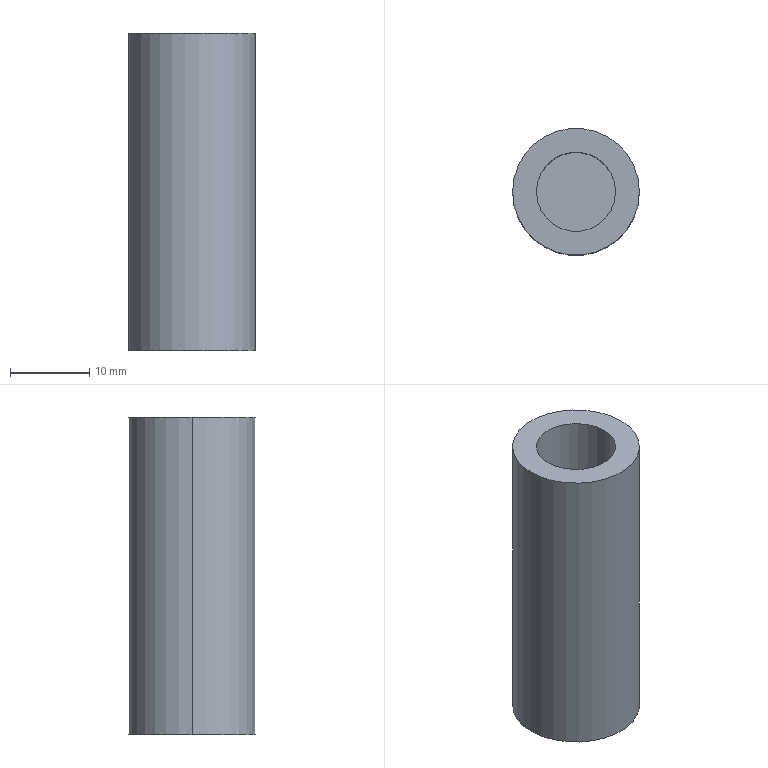Part | SolidWorks | features Extrusion 1, ICE 1 | 1 solid | 7 faces | box 16 x 16 x 40 mm | volume 5451 mm3 | cylinder 4 | plane 3 | commonest cylinder face diameters 10 x2 16 x2
STEP:
#1=CARTESIAN_POINT('',(-5.,0.,7.));
#2=VERTEX_POINT('',#1);
#3=CARTESIAN_POINT('',(5.,0.,7.));
#4=VERTEX_POINT('',#3);
#5=CARTESIAN_POINT('',(0.,0.,7.));
#6=DIRECTION('',(0.,0.,1.));
#7=DIRECTION('',(1.,0.,0.));
#8=AXIS2_PLACEMENT_3D('',#5,#6,#7);
#9=CIRCLE('',#8,5.);
#10=EDGE_CURVE('',#2,#4,#9,.T.);
#11=ORIENTED_EDGE('',*,*,#10,.F.);
#12=CARTESIAN_POINT('',(-5.,0.,40.));
#13=VERTEX_POINT('',#12);
#14=CARTESIAN_POINT('',(-5.,0.,7.));
#15=DIRECTION('',(0.,0.,1.));
#16=VECTOR('',#15,1000.);
#17=LINE('',#14,#16);
#18=EDGE_CURVE('',#2,#13,#17,.T.);
#19=ORIENTED_EDGE('',*,*,#18,.T.);
#20=CARTESIAN_POINT('',(5.,0.,40.));
#21=VERTEX_POINT('',#20);
#22=CARTESIAN_POINT('',(0.,0.,40.));
#23=DIRECTION('',(0.,0.,1.));
#24=DIRECTION('',(1.,0.,0.));
#25=AXIS2_PLACEMENT_3D('',#22,#23,#24);
#26=CIRCLE('',#25,5.);
#27=EDGE_CURVE('',#13,#21,#26,.T.);
#28=ORIENTED_EDGE('',*,*,#27,.T.);
#29=CARTESIAN_POINT('',(5.,0.,7.));
#30=DIRECTION('',(0.,0.,1.));
#31=VECTOR('',#30,1000.);
#32=LINE('',#29,#31);
#33=EDGE_CURVE('',#4,#21,#32,.T.);
#34=ORIENTED_EDGE('',*,*,#33,.F.);
#35=EDGE_LOOP('',(#11,#19,#28,#34));
#36=FACE_OUTER_BOUND('',#35,.T.);
#37=CARTESIAN_POINT('',(0.,0.,7.));
#38=DIRECTION('',(0.,0.,1.));
#39=DIRECTION('',(1.,0.,0.));
#40=AXIS2_PLACEMENT_3D('',#37,#38,#39);
#41=CYLINDRICAL_SURFACE('',#40,5.);
#42=ADVANCED_FACE('',(#36),#41,.F.);
#43=CARTESIAN_POINT('',(8.,0.,40.));
#44=VERTEX_POINT('',#43);
#45=CARTESIAN_POINT('',(-8.,0.,40.));
#46=VERTEX_POINT('',#45);
#47=CARTESIAN_POINT('',(0.,0.,40.));
#48=DIRECTION('',(0.,0.,1.));
#49=DIRECTION('',(1.,0.,0.));
#50=AXIS2_PLACEMENT_3D('',#47,#48,#49);
#51=CIRCLE('',#50,8.);
#52=EDGE_CURVE('',#44,#46,#51,.T.);
#53=ORIENTED_EDGE('',*,*,#52,.F.);
#54=CARTESIAN_POINT('',(8.,0.,0.));
#55=VERTEX_POINT('',#54);
#56=CARTESIAN_POINT('',(8.,0.,40.));
#57=DIRECTION('',(0.,0.,-1.));
#58=VECTOR('',#57,1000.);
#59=LINE('',#56,#58);
#60=EDGE_CURVE('',#44,#55,#59,.T.);
#61=ORIENTED_EDGE('',*,*,#60,.T.);
#62=CARTESIAN_POINT('',(-8.,0.,0.));
#63=VERTEX_POINT('',#62);
#64=CARTESIAN_POINT('',(0.,0.,0.));
#65=DIRECTION('',(0.,0.,1.));
#66=DIRECTION('',(1.,0.,0.));
#67=AXIS2_PLACEMENT_3D('',#64,#65,#66);
#68=CIRCLE('',#67,8.);
#69=EDGE_CURVE('',#55,#63,#68,.T.);
#70=ORIENTED_EDGE('',*,*,#69,.T.);
#71=CARTESIAN_POINT('',(-8.,0.,40.));
#72=DIRECTION('',(0.,0.,-1.));
#73=VECTOR('',#72,1000.);
#74=LINE('',#71,#73);
#75=EDGE_CURVE('',#46,#63,#74,.T.);
#76=ORIENTED_EDGE('',*,*,#75,.F.);
#77=EDGE_LOOP('',(#53,#61,#70,#76));
#78=FACE_OUTER_BOUND('',#77,.T.);
#79=CARTESIAN_POINT('',(0.,0.,40.));
#80=DIRECTION('',(0.,0.,-1.));
#81=DIRECTION('',(-1.,0.,0.));
#82=AXIS2_PLACEMENT_3D('',#79,#80,#81);
#83=CYLINDRICAL_SURFACE('',#82,8.);
#84=ADVANCED_FACE('',(#78),#83,.T.);
#85=ORIENTED_EDGE('',*,*,#60,.F.);
#86=CARTESIAN_POINT('',(0.,0.,40.));
#87=DIRECTION('',(0.,0.,1.));
#88=DIRECTION('',(1.,0.,0.));
#89=AXIS2_PLACEMENT_3D('',#86,#87,#88);
#90=CIRCLE('',#89,8.);
#91=EDGE_CURVE('',#46,#44,#90,.T.);
#92=ORIENTED_EDGE('',*,*,#91,.F.);
#93=ORIENTED_EDGE('',*,*,#75,.T.);
#94=CARTESIAN_POINT('',(0.,0.,0.));
#95=DIRECTION('',(0.,0.,1.));
#96=DIRECTION('',(1.,0.,0.));
#97=AXIS2_PLACEMENT_3D('',#94,#95,#96);
#98=CIRCLE('',#97,8.);
#99=EDGE_CURVE('',#63,#55,#98,.T.);
#100=ORIENTED_EDGE('',*,*,#99,.T.);
#101=EDGE_LOOP('',(#85,#92,#93,#100));
#102=FACE_OUTER_BOUND('',#101,.T.);
#103=CARTESIAN_POINT('',(0.,0.,40.));
#104=DIRECTION('',(0.,0.,-1.));
#105=DIRECTION('',(-1.,0.,0.));
#106=AXIS2_PLACEMENT_3D('',#103,#104,#105);
#107=CYLINDRICAL_SURFACE('',#106,8.);
#108=ADVANCED_FACE('',(#102),#107,.T.);
#109=CARTESIAN_POINT('',(0.,0.,40.));
#110=DIRECTION('',(0.,0.,1.));
#111=DIRECTION('',(1.,0.,0.));
#112=AXIS2_PLACEMENT_3D('',#109,#110,#111);
#113=CIRCLE('',#112,5.);
#114=EDGE_CURVE('',#21,#13,#113,.T.);
#115=ORIENTED_EDGE('',*,*,#114,.F.);
#116=ORIENTED_EDGE('',*,*,#27,.F.);
#117=EDGE_LOOP('',(#115,#116));
#118=FACE_BOUND('',#117,.T.);
#119=ORIENTED_EDGE('',*,*,#91,.T.);
#120=ORIENTED_EDGE('',*,*,#52,.T.);
#121=EDGE_LOOP('',(#119,#120));
#122=FACE_OUTER_BOUND('',#121,.T.);
#123=CARTESIAN_POINT('',(0.,0.,40.));
#124=DIRECTION('',(0.,0.,1.));
#125=DIRECTION('',(1.,0.,0.));
#126=AXIS2_PLACEMENT_3D('',#123,#124,#125);
#127=PLANE('',#126);
#128=ADVANCED_FACE('',(#118,#122),#127,.T.);
#129=ORIENTED_EDGE('',*,*,#99,.F.);
#130=ORIENTED_EDGE('',*,*,#69,.F.);
#131=EDGE_LOOP('',(#129,#130));
#132=FACE_OUTER_BOUND('',#131,.T.);
#133=CARTESIAN_POINT('',(0.,0.,0.));
#134=DIRECTION('',(0.,0.,1.));
#135=DIRECTION('',(1.,0.,0.));
#136=AXIS2_PLACEMENT_3D('',#133,#134,#135);
#137=PLANE('',#136);
#138=ADVANCED_FACE('',(#132),#137,.F.);
#139=ORIENTED_EDGE('',*,*,#18,.F.);
#140=CARTESIAN_POINT('',(0.,0.,7.));
#141=DIRECTION('',(0.,0.,1.));
#142=DIRECTION('',(1.,0.,0.));
#143=AXIS2_PLACEMENT_3D('',#140,#141,#142);
#144=CIRCLE('',#143,5.);
#145=EDGE_CURVE('',#4,#2,#144,.T.);
#146=ORIENTED_EDGE('',*,*,#145,.F.);
#147=ORIENTED_EDGE('',*,*,#33,.T.);
#148=ORIENTED_EDGE('',*,*,#114,.T.);
#149=EDGE_LOOP('',(#139,#146,#147,#148));
#150=FACE_OUTER_BOUND('',#149,.T.);
#151=CARTESIAN_POINT('',(0.,0.,7.));
#152=DIRECTION('',(0.,0.,1.));
#153=DIRECTION('',(1.,0.,0.));
#154=AXIS2_PLACEMENT_3D('',#151,#152,#153);
#155=CYLINDRICAL_SURFACE('',#154,5.);
#156=ADVANCED_FACE('',(#150),#155,.F.);
#157=ORIENTED_EDGE('',*,*,#145,.T.);
#158=ORIENTED_EDGE('',*,*,#10,.T.);
#159=EDGE_LOOP('',(#157,#158));
#160=FACE_OUTER_BOUND('',#159,.T.);
#161=CARTESIAN_POINT('',(0.,0.,7.));
#162=DIRECTION('',(0.,0.,1.));
#163=DIRECTION('',(1.,0.,0.));
#164=AXIS2_PLACEMENT_3D('',#161,#162,#163);
#165=PLANE('',#164);
#166=ADVANCED_FACE('',(#160),#165,.T.);
#167=CLOSED_SHELL('',(#42,#84,#108,#128,#138,#156,#166));
#168=MANIFOLD_SOLID_BREP('',#167);
#169=CARTESIAN_POINT('',(0.,0.,0.));
#170=DIRECTION('',(0.,0.,1.));
#171=DIRECTION('',(1.,0.,0.));
#172=AXIS2_PLACEMENT_3D('',#169,#170,#171);
#173=(LENGTH_UNIT()NAMED_UNIT(*)SI_UNIT(.MILLI.,.METRE.));
#174=UNCERTAINTY_MEASURE_WITH_UNIT(LENGTH_MEASURE(0.00001),#173,'','');
#175=(NAMED_UNIT(*)PLANE_ANGLE_UNIT()SI_UNIT($,.RADIAN.));
#176=(NAMED_UNIT(*)SI_UNIT($,.STERADIAN.)SOLID_ANGLE_UNIT());
#177=(GEOMETRIC_REPRESENTATION_CONTEXT(3)GLOBAL_UNCERTAINTY_ASSIGNED_CONTEXT((#174))GLOBAL_UNIT_ASSIGNED_CONTEXT((#173,#175,#176))REPRESENTATION_CONTEXT('',''));
#178=ADVANCED_BREP_SHAPE_REPRESENTATION('',(#168,#172),#177);